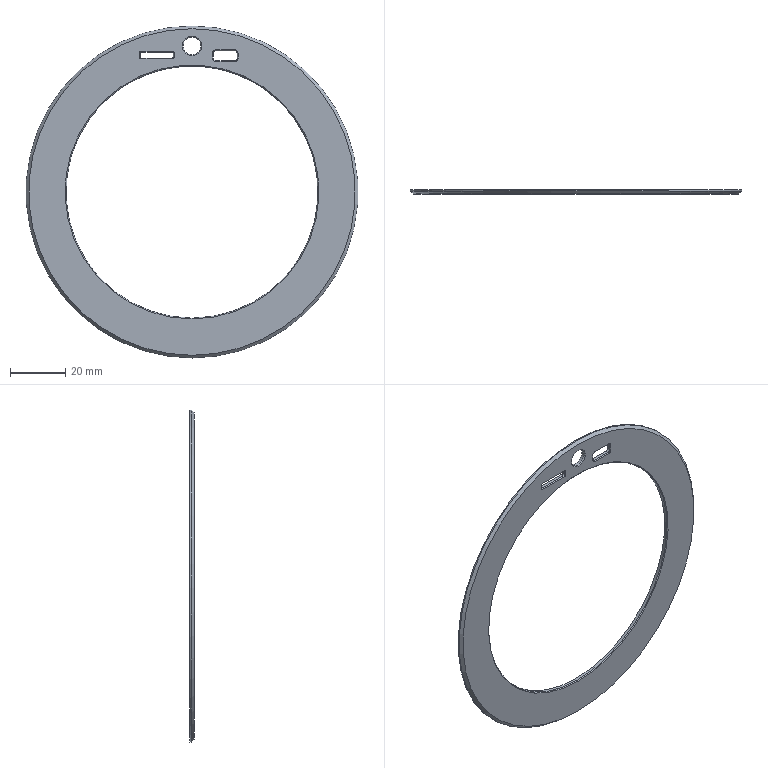NC program | NX | posted with a generic post | part box 119.8 x 1.45 x 119.8 mm
Whole program:
N10 G17 G21 G94 G90
(PROFILE_3D , TOOL : C5.0)
N12 T02 M6
N14 G54
N16 G17 G0 G90 X30.821 Y-57.114 S5000 M3
N18 G43 Z-0.5 H2
N20 G94 G1 Z-1.5 F560.
N22 G41 X29.939 Y-55.354 D2
N24 G3 X27.256 Y-54.46 R2.
N26 G2 X-54.46 Y-27.256 R60.9 F700.
N28 X27.256 Y-54.46 R-60.9
N30 G1 X23.232 Y-56.474
N32 G40
N34 X24.31 Y-59.095
N36 Z1.
(PROFILE_3D_COPY , TOOL : C5.0)
N38 G0 X15.912 Y-36.264 S7000
N40 Z-0.2
N42 G1 Z-1.2 F1500.
N44 G41 X16.83 Y-38.096
N46 G3 X19.513 Y-38.99 R2.
N48 X38.99 Y19.513 R43.6
N50 X19.513 Y-38.99 R-43.6
N52 X20.407 Y-36.306 R2.
N54 G1 X19.937 Y-35.368
N56 G40
N58 X19.489 Y-34.473
N60 Z-0.2
N62 M5
(PROFILE_3D_COPY_COPY , TOOL : C3.0)
N64 T03 M6
N66 G54
N68 G17 G0 G90 X-10.676 Y-48.85 S7000 M3
N70 G43 Z-0.3 H3
N72 G94 G1 Z-0.8 F1500.
N74 G41 Y-48.05 D3
N76 X-15.33
N78 G3 X-15.63 Y-48.35 R0.3
N80 G1 Y-50.05
N82 G3 X-15.33 Y-50.35 R0.3
N84 G1 X-8.6
N86 G3 X-8.3 Y-50.05 R0.3
N88 G1 Y-48.35
N90 G3 X-8.6 Y-48.05 R0.3
N92 G1 X-10.676
N94 G40
N96 X-11.176
N98 Z-0.3
(PROFILE_3D_COPY_COPY_COPY , TOOL : C3.0)
N100 G0 Z0.2
N102 X0. Y-54.2
N104 G1 Z-0.8
N106 G41 Y-55.2
N108 G3 X2.5 Y-52.7 R2.5
N110 X0. Y-55.2 R-2.5
N112 G40
N114 G1 X0.007 Y-54.014
N116 Z0.2
(PROFILE_3D_COPY_COPY_COPY_COPY , TOOL : C3.0)
N118 G0 X13.232 Y-49.117
N120 G1 Z-0.8
N122 G41 X12.74 Y-49.03
N124 X7.44
N126 Y-49.68
N128 X18.04
N130 Y-49.03
N132 X12.74
N134 G40
N136 X12.248 Y-49.117
N138 Z0.2
N140 M5
N142 M2